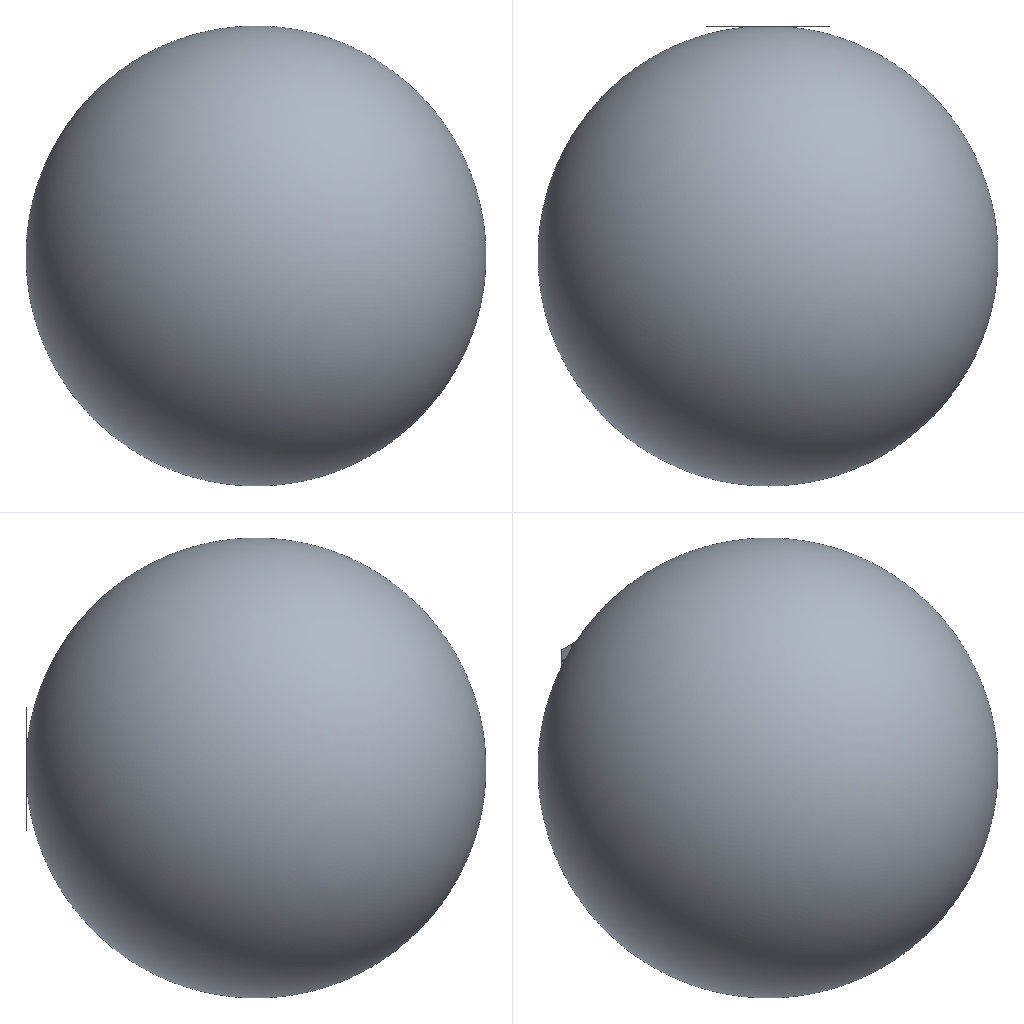Simulation study | abaqus
Set-up summary:
category,name,step,type,value,unit,region
solver,abaqus
solver,version,,,Abaqus/Explicit 2020
units,not stated in the deck,,not stated
analysis,deck,,transient,transient
load_step,Step-1,Step-1,transient
load_step,Step-2,Step-2,transient
load_step,requested,,,2
mesh,nodes,,,59214
mesh,elements,,,57221
element_type,S4R,,shell,57221
load,load commands in deck,,count,2
bc,support commands in deck,,count,2
material,PLATE,,in results
material,SPHERE,,in results
check,setup vs results,,match,"per instance, exact: element labels, types and connectivity; labels of the nodes the elements use; coordinates of those nodes at SINGLE_PRECISION in 2 of 2 instance(s)"
Abaqus input file, long lists of numbers shortened:
*Heading
** Job name: Leng Model name: Model-1
** Generated by: Abaqus/CAE 2020
*Preprint, echo=NO, model=NO, history=NO, contact=NO
**
** PARTS
**
*Part, name=P1
*Node
      1,       10200.,   2774.615,           0.
      2,       10200.,   2579.231,           0.
** (20604 more lines like these left out)
*Element, type=S4R
    1,     6, 17920, 17962,   458
    2,  7507, 17963, 17962, 17920
** (18613 more lines like these left out)
*Nset, nset=Set-1, generate
     1,  20606,      1
*Elset, elset=Set-1, generate
     1,  18615,      1
** Section: plate
*Shell Section, elset=Set-1, material=plate
0.5, 5
*End Part
**
*Part, name=Part-2
*Node
      1,   500.22,   24994.994,           0.
      2,   1499.86,   24954.969,           0.
** (38606 more lines like these left out)
*Element, type=S4R
    1,  3706, 37952,  3783, 38118
    2,  3884,  4086,  3925, 37845
** (38604 more lines like these left out)
*Nset, nset=Set-1, generate
     1,  38608,      1
*Elset, elset=Set-1, generate
     1,  38606,      1
** Section: sphere
*Shell Section, elset=Set-1, material=sphere
1., 5
*End Part
**
**
** ASSEMBLY
**
*Assembly, name=Assembly
**
*Instance, name=Part-2-1, part=Part-2
*End Instance
**
*Instance, name=P1-1, part=P1
      -8400.,       25000.,       -8500.
      -8400.,       25000.,       -8500., -8399.,       25000.,       -8500., 90.
*End Instance
**
*Node
      1, 1.53080847e-12,      -25000.,           0.
*Node
      2,           0.,       25000.,        -200.
*Nset, nset=Set-3
 1,
*Nset, nset=Set-4, instance=Part-2-1, generate
     1,  38608,      1
*Elset, elset=Set-4, instance=Part-2-1, generate
     1,  38606,      1
*Nset, nset=Set-5, instance=Part-2-1, generate
     1,  38608,      1
*Elset, elset=Set-5, instance=Part-2-1, generate
     1,  38606,      1
*Nset, nset=Set-6
 1,
*Nset, nset=Set-7, instance=Part-2-1, generate
     1,  38608,      1
*Nset, nset=Set-7
 1,
*Elset, elset=Set-7, instance=Part-2-1, generate
     1,  38606,      1
*Nset, nset=Set-9
 1,
*Nset, nset=Set-10, instance=Part-2-1, generate
     1,  38608,      1
*Nset, nset=Set-10
 1,
*Elset, elset=Set-10, instance=Part-2-1, generate
     1,  38606,      1
*Nset, nset=Set-12
 2,
*Nset, nset=Set-13, instance=P1-1
  918,  920,  921,  923, 1378, 1379, 1380, 1382
*Nset, nset=Set-14, instance=P1-1
  918,  919,  920,  921,  922,  923, 1377, 1378, 1379, 1380, 1381, 1382
*Elset, elset=Set-14, instance=P1-1
  2720,  2722,  3646,  7844,  8385,  8429,  8437,  8472,  8548, 17818
*Nset, nset=m_Set-1
 1,
*Nset, nset=m_Set-8
 1,
*Nset, nset=m_Set-11
 2,
*Nset, nset=s_Set-2, instance=Part-2-1
 105,
*Elset, elset=_Surf-3_SNEG, internal, instance=P1-1, generate
     1,  18615,      1
*Surface, type=ELEMENT, name=Surf-3
_Surf-3_SNEG, SNEG
*Elset, elset=_Surf-4_SNEG, internal, instance=Part-2-1, generate
     1,  38606,      1
*Surface, type=ELEMENT, name=Surf-4
_Surf-4_SNEG, SNEG
*Elset, elset=_Surf-7_SNEG, internal, instance=P1-1, generate
     1,  18615,      1
*Surface, type=ELEMENT, name=Surf-7
_Surf-7_SNEG, SNEG
*Elset, elset=_Surf-8_SNEG, internal, instance=Part-2-1, generate
     1,  38606,      1
*Surface, type=ELEMENT, name=Surf-8
_Surf-8_SNEG, SNEG
*Elset, elset=_Surf-15_SNEG, internal, instance=Part-2-1, generate
     1,  38606,      1
*Surface, type=ELEMENT, name=Surf-15
_Surf-15_SNEG, SNEG
*Elset, elset=_m_Surf-2_SPOS, internal, instance=Part-2-1, generate
     1,  38606,      1
*Surface, type=ELEMENT, name=m_Surf-2
_m_Surf-2_SPOS, SPOS
*Elset, elset=_m_Surf-5_SPOS, internal, instance=P1-1, generate
     1,  18615,      1
*Surface, type=ELEMENT, name=m_Surf-5
_m_Surf-5_SPOS, SPOS
*Elset, elset=_m_Surf-10_SPOS, internal, instance=Part-2-1, generate
     1,  38606,      1
*Surface, type=ELEMENT, name=m_Surf-10
_m_Surf-10_SPOS, SPOS
*Elset, elset=_m_Surf-12_SPOS, internal, instance=P1-1, generate
     1,  18615,      1
*Surface, type=ELEMENT, name=m_Surf-12
_m_Surf-12_SPOS, SPOS
*Elset, elset=_s_Surf-1_SPOS, internal, instance=Part-2-1, generate
     1,  38606,      1
*Surface, type=ELEMENT, name=s_Surf-1
_s_Surf-1_SPOS, SPOS
*Elset, elset=_s_Surf-5_SPOS, internal, instance=Part-2-1, generate
     1,  38606,      1
*Surface, type=ELEMENT, name=s_Surf-5
_s_Surf-5_SPOS, SPOS
*Elset, elset=_s_Surf-9_SPOS, internal, instance=Part-2-1, generate
     1,  38606,      1
*Surface, type=ELEMENT, name=s_Surf-9
_s_Surf-9_SPOS, SPOS
*Elset, elset=_s_Surf-10_SPOS, internal, instance=P1-1, generate
     1,  18615,      1
*Surface, type=ELEMENT, name=s_Surf-10
_s_Surf-10_SPOS, SPOS
*Elset, elset=_s_Surf-12_SPOS, internal, instance=Part-2-1, generate
     1,  38606,      1
*Surface, type=ELEMENT, name=s_Surf-12
_s_Surf-12_SPOS, SPOS
*Elset, elset=_s_Surf-14_SNEG, internal, instance=P1-1, generate
     1,  18615,      1
*Surface, type=ELEMENT, name=s_Surf-14
_s_Surf-14_SNEG, SNEG
*End Assembly
*Amplitude, name=Amp-1
             0.,              0.,           0.001,              1.
**
** MATERIALS
**
*Material, name=plate
*Density
 1e-09,
*Elastic
1000., 0.4
*Material, name=sphere
*Density
 7e-09,
*Elastic
200000., 0.3
**
** INTERACTION PROPERTIES
**
*Surface Interaction, name=IntProp-1
*Friction
 0.2,
*Surface Behavior, pressure-overclosure=HARD
** ----------------------------------------------------------------
**
** STEP: Step-1
**
*Step, name=Step-1, nlgeom=YES
*Dynamic, Explicit
, 0.1
*Bulk Viscosity
0.06, 1.2
** Mass Scaling: Semi-Automatic
**               Whole Model
*Fixed Mass Scaling, factor=5000.
**
** BOUNDARY CONDITIONS
**
** Name: BC-1 Type: 对称/反对称/完全固定
*Boundary
Set-10, ENCASTRE
**
** LOADS
**
** Name: Load-1   Type: Pressure
*Dsload, amplitude=Amp-1
Surf-7, P, 1.
**
** INTERACTIONS
**
** Interaction: Int-2
*Contact Pair, interaction=IntProp-1, mechanical constraint=KINEMATIC, cpset=Int-2
m_Surf-12, s_Surf-12
**
** OUTPUT REQUESTS
**
*Restart, write, number interval=1, time marks=NO
**
** FIELD OUTPUT: F-Output-1
**
*Output, field
*Node Output
A, CF, RF, U, V
*Element Output, directions=YES
LE, MISES, MISESMAX, PE, PEEQ, PEMAG, S, SSAVG
*Contact Output
CDISP, CSTRESS
**
** HISTORY OUTPUT: H-Output-1
**
*Output, history, variable=PRESELECT
*End Step
** ----------------------------------------------------------------
**
** STEP: Step-2
**
*Step, name=Step-2, nlgeom=YES
*Dynamic, Explicit
, 0.1
*Bulk Viscosity
0.06, 1.2
** Mass Scaling: Semi-Automatic
**               Whole Model
*Fixed Mass Scaling, factor=500.
**
** BOUNDARY CONDITIONS
**
** Name: BC-1 Type: 对称/反对称/完全固定
*Boundary, op=NEW
** Name: BC-2 Type: 位移/转角
*Boundary, op=NEW
Set-14, 2, 2
**
** LOADS
**
** Name: Load-2   Type: Pressure
*Dsload, amplitude=Amp-1
Surf-15, P, 1.
**
** OUTPUT REQUESTS
**
*Restart, write, number interval=1, time marks=NO
**
** FIELD OUTPUT: F-Output-1
**
*Output, field
*Node Output
A, CF, RF, U, V
*Element Output, directions=YES
LE, MISES, MISESMAX, PE, PEEQ, PEMAG, S, SSAVG
*Contact Output
CDISP, CSTRESS
**
** HISTORY OUTPUT: H-Output-1
**
*Output, history, variable=PRESELECT
*End Step
Results summary:
result,step,Step-1,completed,increments=63 time=0.1/0.1
result,step,Step-2,completed,increments=194 time=0.1/0.1
result,analysis,,,transient
result,last_loadstep,,,2
result,primary field,,,"U, UR"
result,reaction total,,FX,0.0,model units
result,reaction total,,FY,-2018326.531,model units
result,reaction total,,FZ,0.0,model units